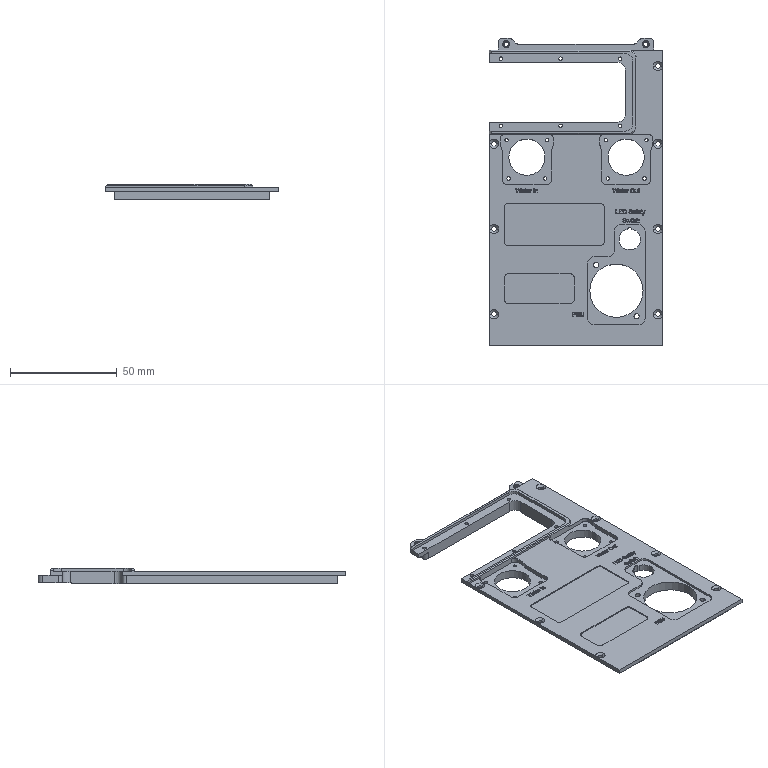NC program | NX | posted with a generic post | part box 81.5 x 144.28 x 7.5 mm
Lines 7294 to 9048 of 9048:
(CAVITY_MILL_COPY_COPY , TOOL : D2精光)
N14478 T10 M6
N14480 G54
N14482 G17 G0 G90 X29.54 Y-11.576 S6500 M3
N14484 G43 Z50. H10
N14486 Z0.
N14488 G94 G1 Z-0.2 F1200.
N14490 G3 X29.74 Y-11.376 R0.2
N14492 G1 Y-10.85
N14494 X29.602
N14496 G2 X29.301 Y-10.828 R2.1
N14498 G3 X29.076 Y-10.989 R0.2
N14500 G1 Z0.
N14502 G0 X29.54 Y-11.576 Z-0.2
N14504 G1 Z-0.4
N14506 G3 X29.74 Y-11.376 R0.2
N14508 G1 Y-10.85
N14510 X29.602
N14512 G2 X29.301 Y-10.828 R2.1
N14514 G3 X29.076 Y-10.989 R0.2
N14516 G1 Z-0.2
N14518 G0 X29.54 Y-11.576 Z-0.388
N14520 G1 Z-0.588
N14522 G3 X29.74 Y-11.376 R0.2
N14524 G1 Y-10.85
N14526 X29.602
N14528 G2 X29.301 Y-10.828 R2.1
N14530 G3 X29.076 Y-10.989 R0.2
N14532 G1 Z-0.388
N14534 G0 X29.54 Y-11.576 Z-0.575
N14536 G1 Z-0.775
N14538 G3 X29.74 Y-11.376 R0.2
N14540 G1 Y-10.85
N14542 X29.602
N14544 G2 X29.301 Y-10.828 R2.1
N14546 G3 X29.076 Y-10.989 R0.2
N14548 G1 Z-0.575
N14550 G0 X29.54 Y-11.576 Z-0.763
N14552 G1 Z-0.963
N14554 G3 X29.74 Y-11.376 R0.2
N14556 G1 Y-10.85
N14558 X29.602
N14560 G2 X29.301 Y-10.828 R2.1
N14562 G3 X29.076 Y-10.989 R0.2
N14564 G1 Z-0.763
N14566 G0 X29.54 Y-11.576 Z-0.95
N14568 G1 Z-1.15
N14570 G3 X29.74 Y-11.376 R0.2
N14572 G1 Y-10.85
N14574 X29.602
N14576 G2 X29.301 Y-10.828 R2.1
N14578 G3 X29.076 Y-10.989 R0.2
N14580 G1 Z-0.95
N14582 G0 X29.54 Y-11.576 Z-1.138
N14584 G1 Z-1.338
N14586 G3 X29.74 Y-11.376 R0.2
N14588 G1 Y-10.85
N14590 X29.602
N14592 G2 X29.301 Y-10.828 R2.1
N14594 G3 X29.076 Y-10.989 R0.2
N14596 G1 Z-1.138
N14598 G0 X29.54 Y-11.576 Z-1.325
N14600 G1 Z-1.525
N14602 G3 X29.74 Y-11.376 R0.2
N14604 G1 Y-10.85
N14606 X29.602
N14608 G2 X29.301 Y-10.828 R2.1
N14610 G3 X29.076 Y-10.989 R0.2
N14612 G1 Z-1.325
N14614 G0 X29.54 Y-11.576 Z-1.513
N14616 G1 Z-1.713
N14618 G3 X29.74 Y-11.376 R0.2
N14620 G1 Y-10.85
N14622 X29.602
N14624 G2 X29.301 Y-10.828 R2.1
N14626 G3 X29.076 Y-10.989 R0.2
N14628 G1 Z-1.513
N14630 G0 X29.54 Y-11.576 Z-1.7
N14632 G1 Z-1.9
N14634 G3 X29.74 Y-11.376 R0.2
N14636 G1 Y-10.85
N14638 X29.602
N14640 G2 X29.301 Y-10.828 R2.1
N14642 G3 X29.076 Y-10.989 R0.2
N14644 G1 Z-1.7
N14646 G0 X29.54 Y-11.576 Z-1.9
N14648 G1 Z-2.1
N14650 G3 X29.74 Y-11.376 R0.2
N14652 G1 Y-10.85
N14654 X29.602
N14656 G2 X29.301 Y-10.828 R2.1
N14658 G3 X29.076 Y-10.989 R0.2
N14660 G1 Z-1.9
N14662 G0 X29.54 Y-11.576 Z-2.1
N14664 G1 Z-2.3
N14666 G3 X29.74 Y-11.376 R0.2
N14668 G1 Y-10.85
N14670 X29.602
N14672 G2 X29.301 Y-10.828 R2.1
N14674 G3 X29.076 Y-10.989 R0.2
N14676 G1 Z-2.1
N14678 G0 X29.54 Y-11.576 Z-2.3
N14680 G1 Z-2.5
N14682 G3 X29.74 Y-11.376 R0.2
N14684 G1 Y-10.85
N14686 X29.602
N14688 G2 X29.301 Y-10.828 R2.1
N14690 G3 X29.076 Y-10.989 R0.2
N14692 G1 Z-2.3
N14694 G0 X29.54 Y-11.576 Z-2.5
N14696 G1 Z-2.7
N14698 G3 X29.74 Y-11.376 R0.2
N14700 G1 Y-10.85
N14702 X29.602
N14704 G2 X29.301 Y-10.828 R2.1
N14706 G3 X29.076 Y-10.989 R0.2
N14708 G1 Z-2.5
N14710 G0 X29.54 Y-11.576 Z-2.7
N14712 G1 Z-2.9
N14714 G3 X29.74 Y-11.376 R0.2
N14716 G1 Y-10.85
N14718 X29.602
N14720 G2 X29.301 Y-10.828 R2.1
N14722 G3 X29.076 Y-10.989 R0.2
N14724 G1 Z-2.7
N14726 G0 Z50.
N14728 X64.585 Y-10.975
N14730 Z-0.388
N14732 G1 Z-0.588
N14734 G3 X64.356 Y-10.82 R0.2
N14736 G2 X64.002 Y-10.85 R2.1
N14738 G1 X63.94
N14740 Y-11.353
N14742 G3 X64.14 Y-11.553 R0.2
N14744 G1 Z-0.388
N14746 G0 X64.585 Y-10.975 Z-0.575
N14748 G1 Z-0.775
N14750 G3 X64.356 Y-10.82 R0.2
N14752 G2 X64.002 Y-10.85 R2.1
N14754 G1 X63.94
N14756 Y-11.353
N14758 G3 X64.14 Y-11.553 R0.2
N14760 G1 Z-0.575
N14762 G0 X64.585 Y-10.975 Z-0.763
N14764 G1 Z-0.963
N14766 G3 X64.356 Y-10.82 R0.2
N14768 G2 X64.002 Y-10.85 R2.1
N14770 G1 X63.94
N14772 Y-11.353
N14774 G3 X64.14 Y-11.553 R0.2
N14776 G1 Z-0.763
N14778 G0 X64.585 Y-10.975 Z-0.95
N14780 G1 Z-1.15
N14782 G3 X64.356 Y-10.82 R0.2
N14784 G2 X64.002 Y-10.85 R2.1
N14786 G1 X63.94
N14788 Y-11.353
N14790 G3 X64.14 Y-11.553 R0.2
N14792 G1 Z-0.95
N14794 G0 X64.585 Y-10.975 Z-1.138
N14796 G1 Z-1.338
N14798 G3 X64.356 Y-10.82 R0.2
N14800 G2 X64.002 Y-10.85 R2.1
N14802 G1 X63.94
N14804 Y-11.353
N14806 G3 X64.14 Y-11.553 R0.2
N14808 G1 Z-1.138
N14810 G0 X64.585 Y-10.975 Z-1.325
N14812 G1 Z-1.525
N14814 G3 X64.356 Y-10.82 R0.2
N14816 G2 X64.002 Y-10.85 R2.1
N14818 G1 X63.94
N14820 Y-11.353
N14822 G3 X64.14 Y-11.553 R0.2
N14824 G1 Z-1.325
N14826 G0 X64.585 Y-10.975 Z-1.513
N14828 G1 Z-1.713
N14830 G3 X64.356 Y-10.82 R0.2
N14832 G2 X64.002 Y-10.85 R2.1
N14834 G1 X63.94
N14836 Y-11.353
N14838 G3 X64.14 Y-11.553 R0.2
N14840 G1 Z-1.513
N14842 G0 X64.585 Y-10.975 Z-1.7
N14844 G1 Z-1.9
N14846 G3 X64.356 Y-10.82 R0.2
N14848 G2 X64.002 Y-10.85 R2.1
N14850 G1 X63.94
N14852 Y-11.353
N14854 G3 X64.14 Y-11.553 R0.2
N14856 G1 Z-1.7
N14858 G0 X64.585 Y-10.975 Z-1.9
N14860 G1 Z-2.1
N14862 G3 X64.356 Y-10.82 R0.2
N14864 G2 X64.002 Y-10.85 R2.1
N14866 G1 X63.94
N14868 Y-11.353
N14870 G3 X64.14 Y-11.553 R0.2
N14872 G1 Z-1.9
N14874 G0 X64.585 Y-10.975 Z-2.1
N14876 G1 Z-2.3
N14878 G3 X64.356 Y-10.82 R0.2
N14880 G2 X64.002 Y-10.85 R2.1
N14882 G1 X63.94
N14884 Y-11.353
N14886 G3 X64.14 Y-11.553 R0.2
N14888 G1 Z-2.1
N14890 G0 X64.585 Y-10.975 Z-2.3
N14892 G1 Z-2.5
N14894 G3 X64.356 Y-10.82 R0.2
N14896 G2 X64.002 Y-10.85 R2.1
N14898 G1 X63.94
N14900 Y-11.353
N14902 G3 X64.14 Y-11.553 R0.2
N14904 G1 Z-2.3
N14906 G0 X64.585 Y-10.975 Z-2.5
N14908 G1 Z-2.7
N14910 G3 X64.356 Y-10.82 R0.2
N14912 G2 X64.002 Y-10.85 R2.1
N14914 G1 X63.94
N14916 Y-11.353
N14918 G3 X64.14 Y-11.553 R0.2
N14920 G1 Z-2.5
N14922 G0 X64.585 Y-10.975 Z-2.7
N14924 G1 Z-2.9
N14926 G3 X64.356 Y-10.82 R0.2
N14928 G2 X64.002 Y-10.85 R2.1
N14930 G1 X63.94
N14932 Y-11.353
N14934 G3 X64.14 Y-11.553 R0.2
N14936 G1 Z-2.7
N14938 G0 Z50.
N14940 X65.929 Y-4.022
N14942 Z-0.388
N14944 G1 Z-0.588
N14946 X65.94 Y-4.043
N14948 G3 X66.207 Y-4.135 R0.2
N14950 X66.74 Y-3.535 R1.06
N14952 G1 Y-10.965
N14954 G3 X65.407 Y-10.31 R1.06
N14956 X66.102 Y-8.75 R2.1
N14958 G1 Y-5.75
N14960 G3 X65.407 Y-4.19 R2.1
N14962 X66.207 Y-4.135 R1.06
N14964 X66.288 Y-3.846 R0.201
N14966 G1 Z-0.388
N14968 G0 X65.929 Y-4.022 Z-0.575
N14970 G1 Z-0.775
N14972 X65.94 Y-4.043
N14974 G3 X66.207 Y-4.135 R0.2
N14976 X66.74 Y-3.535 R1.06
N14978 G1 Y-10.965
N14980 G3 X65.407 Y-10.31 R1.06
N14982 X66.102 Y-8.75 R2.1
N14984 G1 Y-5.75
N14986 G3 X65.407 Y-4.19 R2.1
N14988 X66.207 Y-4.135 R1.06
N14990 X66.288 Y-3.846 R0.201
N14992 G1 Z-0.575
N14994 G0 X65.929 Y-4.022 Z-0.763
N14996 G1 Z-0.963
N14998 X65.94 Y-4.043
N15000 G3 X66.207 Y-4.135 R0.2
N15002 X66.74 Y-3.535 R1.06
N15004 G1 Y-10.965
N15006 G3 X65.407 Y-10.31 R1.06
N15008 X66.102 Y-8.75 R2.1
N15010 G1 Y-5.75
N15012 G3 X65.407 Y-4.19 R2.1
N15014 X66.207 Y-4.135 R1.06
N15016 X66.288 Y-3.846 R0.201
N15018 G1 Z-0.763
N15020 G0 X65.929 Y-4.022 Z-0.95
N15022 G1 Z-1.15
N15024 X65.94 Y-4.043
N15026 G3 X66.207 Y-4.135 R0.2
N15028 X66.74 Y-3.535 R1.06
N15030 G1 Y-10.965
N15032 G3 X65.407 Y-10.31 R1.06
N15034 X66.102 Y-8.75 R2.1
N15036 G1 Y-5.75
N15038 G3 X65.407 Y-4.19 R2.1
N15040 X66.207 Y-4.135 R1.06
N15042 X66.288 Y-3.846 R0.201
N15044 G1 Z-0.95
N15046 G0 X65.929 Y-4.022 Z-1.138
N15048 G1 Z-1.338
N15050 X65.94 Y-4.043
N15052 G3 X66.207 Y-4.135 R0.2
N15054 X66.74 Y-3.535 R1.06
N15056 G1 Y-10.965
N15058 G3 X65.407 Y-10.31 R1.06
N15060 X66.102 Y-8.75 R2.1
N15062 G1 Y-5.75
N15064 G3 X65.407 Y-4.19 R2.1
N15066 X66.207 Y-4.135 R1.06
N15068 X66.288 Y-3.846 R0.201
N15070 G1 Z-1.138
N15072 G0 X65.929 Y-4.022 Z-1.325
N15074 G1 Z-1.525
N15076 X65.94 Y-4.043
N15078 G3 X66.207 Y-4.135 R0.2
N15080 X66.74 Y-3.535 R1.06
N15082 G1 Y-10.965
N15084 G3 X65.407 Y-10.31 R1.06
N15086 X66.102 Y-8.75 R2.1
N15088 G1 Y-5.75
N15090 G3 X65.407 Y-4.19 R2.1
N15092 X66.207 Y-4.135 R1.06
N15094 X66.288 Y-3.846 R0.201
N15096 G1 Z-1.325
N15098 G0 X65.929 Y-4.022 Z-1.513
N15100 G1 Z-1.713
N15102 X65.94 Y-4.043
N15104 G3 X66.207 Y-4.135 R0.2
N15106 X66.74 Y-3.535 R1.06
N15108 G1 Y-10.965
N15110 G3 X65.407 Y-10.31 R1.06
N15112 X66.102 Y-8.75 R2.1
N15114 G1 Y-5.75
N15116 G3 X65.407 Y-4.19 R2.1
N15118 X66.207 Y-4.135 R1.06
N15120 X66.288 Y-3.846 R0.201
N15122 G1 Z-1.513
N15124 G0 X65.929 Y-4.022 Z-1.7
N15126 G1 Z-1.9
N15128 X65.94 Y-4.043
N15130 G3 X66.207 Y-4.135 R0.2
N15132 X66.74 Y-3.535 R1.06
N15134 G1 Y-10.965
N15136 G3 X65.407 Y-10.31 R1.06
N15138 X66.102 Y-8.75 R2.1
N15140 G1 Y-5.75
N15142 G3 X65.407 Y-4.19 R2.1
N15144 X66.207 Y-4.135 R1.06
N15146 X66.288 Y-3.846 R0.201
N15148 G1 Z-1.7
N15150 G0 X65.929 Y-4.022 Z-1.9
N15152 G1 Z-2.1
N15154 X65.94 Y-4.043
N15156 G3 X66.207 Y-4.135 R0.2
N15158 X66.74 Y-3.535 R1.06
N15160 G1 Y-10.965
N15162 G3 X65.407 Y-10.31 R1.06
N15164 X66.102 Y-8.75 R2.1
N15166 G1 Y-5.75
N15168 G3 X65.407 Y-4.19 R2.1
N15170 X66.207 Y-4.135 R1.06
N15172 X66.288 Y-3.846 R0.201
N15174 G1 Z-1.9
N15176 G0 X65.929 Y-4.022 Z-2.1
N15178 G1 Z-2.3
N15180 X65.94 Y-4.043
N15182 G3 X66.207 Y-4.135 R0.2
N15184 X66.74 Y-3.535 R1.06
N15186 G1 Y-10.965
N15188 G3 X65.407 Y-10.31 R1.06
N15190 X66.102 Y-8.75 R2.1
N15192 G1 Y-5.75
N15194 G3 X65.407 Y-4.19 R2.1
N15196 X66.207 Y-4.135 R1.06
N15198 X66.288 Y-3.846 R0.201
N15200 G1 Z-2.1
N15202 G0 X65.929 Y-4.022 Z-2.3
N15204 G1 Z-2.5
N15206 X65.94 Y-4.043
N15208 G3 X66.207 Y-4.135 R0.2
N15210 X66.74 Y-3.535 R1.06
N15212 G1 Y-10.965
N15214 G3 X65.407 Y-10.31 R1.06
N15216 X66.102 Y-8.75 R2.1
N15218 G1 Y-5.75
N15220 G3 X65.407 Y-4.19 R2.1
N15222 X66.207 Y-4.135 R1.06
N15224 X66.288 Y-3.846 R0.201
N15226 G1 Z-2.3
N15228 G0 X65.929 Y-4.022 Z-2.5
N15230 G1 Z-2.7
N15232 X65.94 Y-4.043
N15234 G3 X66.207 Y-4.135 R0.2
N15236 X66.74 Y-3.535 R1.06
N15238 G1 Y-10.965
N15240 G3 X65.407 Y-10.31 R1.06
N15242 X66.102 Y-8.75 R2.1
N15244 G1 Y-5.75
N15246 G3 X65.407 Y-4.19 R2.1
N15248 X66.207 Y-4.135 R1.06
N15250 X66.288 Y-3.846 R0.201
N15252 G1 Z-2.5
N15254 G0 X65.929 Y-4.022 Z-2.7
N15256 G1 Z-2.9
N15258 X65.94 Y-4.043
N15260 G3 X66.207 Y-4.135 R0.2
N15262 X66.74 Y-3.535 R1.06
N15264 G1 Y-10.965
N15266 G3 X65.407 Y-10.31 R1.06
N15268 X66.102 Y-8.75 R2.1
N15270 G1 Y-5.75
N15272 G3 X65.407 Y-4.19 R2.1
N15274 X66.207 Y-4.135 R1.06
N15276 X66.288 Y-3.846 R0.201
N15278 G1 Z-2.7
N15280 G0 X64.14 Y-2.947 Z-0.388
N15282 G1 Z-0.588
N15284 G3 X63.94 Y-3.147 R0.2
N15286 G1 Y-3.65
N15288 X64.002
N15290 G2 X64.356 Y-3.68 R2.1
N15292 G3 X64.585 Y-3.525 R0.2
N15294 G1 Z-0.388
N15296 G0 X64.14 Y-2.947 Z-0.575
N15298 G1 Z-0.775
N15300 G3 X63.94 Y-3.147 R0.2
N15302 G1 Y-3.65
N15304 X64.002
N15306 G2 X64.356 Y-3.68 R2.1
N15308 G3 X64.585 Y-3.525 R0.2
N15310 G1 Z-0.575
N15312 G0 X64.14 Y-2.947 Z-0.763
N15314 G1 Z-0.963
N15316 G3 X63.94 Y-3.147 R0.2
N15318 G1 Y-3.65
N15320 X64.002
N15322 G2 X64.356 Y-3.68 R2.1
N15324 G3 X64.585 Y-3.525 R0.2
N15326 G1 Z-0.763
N15328 G0 X64.14 Y-2.947 Z-0.95
N15330 G1 Z-1.15
N15332 G3 X63.94 Y-3.147 R0.2
N15334 G1 Y-3.65
N15336 X64.002
N15338 G2 X64.356 Y-3.68 R2.1
N15340 G3 X64.585 Y-3.525 R0.2
N15342 G1 Z-0.95
N15344 G0 X64.14 Y-2.947 Z-1.138
N15346 G1 Z-1.338
N15348 G3 X63.94 Y-3.147 R0.2
N15350 G1 Y-3.65
N15352 X64.002
N15354 G2 X64.356 Y-3.68 R2.1
N15356 G3 X64.585 Y-3.525 R0.2
N15358 G1 Z-1.138
N15360 G0 X64.14 Y-2.947 Z-1.325
N15362 G1 Z-1.525
N15364 G3 X63.94 Y-3.147 R0.2
N15366 G1 Y-3.65
N15368 X64.002
N15370 G2 X64.356 Y-3.68 R2.1
N15372 G3 X64.585 Y-3.525 R0.2
N15374 G1 Z-1.325
N15376 G0 X64.14 Y-2.947 Z-1.513
N15378 G1 Z-1.713
N15380 G3 X63.94 Y-3.147 R0.2
N15382 G1 Y-3.65
N15384 X64.002
N15386 G2 X64.356 Y-3.68 R2.1
N15388 G3 X64.585 Y-3.525 R0.2
N15390 G1 Z-1.513
N15392 G0 X64.14 Y-2.947 Z-1.7
N15394 G1 Z-1.9
N15396 G3 X63.94 Y-3.147 R0.2
N15398 G1 Y-3.65
N15400 X64.002
N15402 G2 X64.356 Y-3.68 R2.1
N15404 G3 X64.585 Y-3.525 R0.2
N15406 G1 Z-1.7
N15408 G0 X64.14 Y-2.947 Z-1.9
N15410 G1 Z-2.1
N15412 G3 X63.94 Y-3.147 R0.2
N15414 G1 Y-3.65
N15416 X64.002
N15418 G2 X64.356 Y-3.68 R2.1
N15420 G3 X64.585 Y-3.525 R0.2
N15422 G1 Z-1.9
N15424 G0 X64.14 Y-2.947 Z-2.1
N15426 G1 Z-2.3
N15428 G3 X63.94 Y-3.147 R0.2
N15430 G1 Y-3.65
N15432 X64.002
N15434 G2 X64.356 Y-3.68 R2.1
N15436 G3 X64.585 Y-3.525 R0.2
N15438 G1 Z-2.1
N15440 G0 X64.14 Y-2.947 Z-2.3
N15442 G1 Z-2.5
N15444 G3 X63.94 Y-3.147 R0.2
N15446 G1 Y-3.65
N15448 X64.002
N15450 G2 X64.356 Y-3.68 R2.1
N15452 G3 X64.585 Y-3.525 R0.2
N15454 G1 Z-2.3
N15456 G0 X64.14 Y-2.947 Z-2.5
N15458 G1 Z-2.7
N15460 G3 X63.94 Y-3.147 R0.2
N15462 G1 Y-3.65
N15464 X64.002
N15466 G2 X64.356 Y-3.68 R2.1
N15468 G3 X64.585 Y-3.525 R0.2
N15470 G1 Z-2.5
N15472 G0 X64.14 Y-2.947 Z-2.7
N15474 G1 Z-2.9
N15476 G3 X63.94 Y-3.147 R0.2
N15478 G1 Y-3.65
N15480 X64.002
N15482 G2 X64.356 Y-3.68 R2.1
N15484 G3 X64.585 Y-3.525 R0.2
N15486 G1 Z-2.7
N15488 G0 X66.288 Y17.346 Z-0.388
N15490 G1 Z-0.588
N15492 X66.299 Y17.367
N15494 G3 X66.207 Y17.635 R0.2
N15496 X65.407 Y17.69 R1.06
N15498 X66.102 Y19.25 R2.1
N15500 G1 Y22.25
N15502 G3 X65.407 Y23.81 R2.1
N15504 X66.74 Y24.465 R1.06
N15506 G1 Y17.035
N15508 G3 X66.207 Y17.635 R1.06
N15510 X65.929 Y17.522 R0.201
N15512 G1 Z-0.388
N15514 G0 X66.288 Y17.346 Z-0.575
N15516 G1 Z-0.775
N15518 X66.299 Y17.367
N15520 G3 X66.207 Y17.635 R0.2
N15522 X65.407 Y17.69 R1.06
N15524 X66.102 Y19.25 R2.1
N15526 G1 Y22.25
N15528 G3 X65.407 Y23.81 R2.1
N15530 X66.74 Y24.465 R1.06
N15532 G1 Y17.035
N15534 G3 X66.207 Y17.635 R1.06
N15536 X65.929 Y17.522 R0.201
N15538 G1 Z-0.575
N15540 G0 X66.288 Y17.346 Z-0.763
N15542 G1 Z-0.963
N15544 X66.299 Y17.367
N15546 G3 X66.207 Y17.635 R0.2
N15548 X65.407 Y17.69 R1.06
N15550 X66.102 Y19.25 R2.1
N15552 G1 Y22.25
N15554 G3 X65.407 Y23.81 R2.1
N15556 X66.74 Y24.465 R1.06
N15558 G1 Y17.035
N15560 G3 X66.207 Y17.635 R1.06
N15562 X65.929 Y17.522 R0.201
N15564 G1 Z-0.763
N15566 G0 X66.288 Y17.346 Z-0.95
N15568 G1 Z-1.15
N15570 X66.299 Y17.367
N15572 G3 X66.207 Y17.635 R0.2
N15574 X65.407 Y17.69 R1.06
N15576 X66.102 Y19.25 R2.1
N15578 G1 Y22.25
N15580 G3 X65.407 Y23.81 R2.1
N15582 X66.74 Y24.465 R1.06
N15584 G1 Y17.035
N15586 G3 X66.207 Y17.635 R1.06
N15588 X65.929 Y17.522 R0.201
N15590 G1 Z-0.95
N15592 G0 X66.288 Y17.346 Z-1.138
N15594 G1 Z-1.338
N15596 X66.299 Y17.367
N15598 G3 X66.207 Y17.635 R0.2
N15600 X65.407 Y17.69 R1.06
N15602 X66.102 Y19.25 R2.1
N15604 G1 Y22.25
N15606 G3 X65.407 Y23.81 R2.1
N15608 X66.74 Y24.465 R1.06
N15610 G1 Y17.035
N15612 G3 X66.207 Y17.635 R1.06
N15614 X65.929 Y17.522 R0.201
N15616 G1 Z-1.138
N15618 G0 X66.288 Y17.346 Z-1.325
N15620 G1 Z-1.525
N15622 X66.299 Y17.367
N15624 G3 X66.207 Y17.635 R0.2
N15626 X65.407 Y17.69 R1.06
N15628 X66.102 Y19.25 R2.1
N15630 G1 Y22.25
N15632 G3 X65.407 Y23.81 R2.1
N15634 X66.74 Y24.465 R1.06
N15636 G1 Y17.035
N15638 G3 X66.207 Y17.635 R1.06
N15640 X65.929 Y17.522 R0.201
N15642 G1 Z-1.325
N15644 G0 X66.288 Y17.346 Z-1.513
N15646 G1 Z-1.713
N15648 X66.299 Y17.367
N15650 G3 X66.207 Y17.635 R0.2
N15652 X65.407 Y17.69 R1.06
N15654 X66.102 Y19.25 R2.1
N15656 G1 Y22.25
N15658 G3 X65.407 Y23.81 R2.1
N15660 X66.74 Y24.465 R1.06
N15662 G1 Y17.035
N15664 G3 X66.207 Y17.635 R1.06
N15666 X65.929 Y17.522 R0.201
N15668 G1 Z-1.513
N15670 G0 X66.288 Y17.346 Z-1.7
N15672 G1 Z-1.9
N15674 X66.299 Y17.367
N15676 G3 X66.207 Y17.635 R0.2
N15678 X65.407 Y17.69 R1.06
N15680 X66.102 Y19.25 R2.1
N15682 G1 Y22.25
N15684 G3 X65.407 Y23.81 R2.1
N15686 X66.74 Y24.465 R1.06
N15688 G1 Y17.035
N15690 G3 X66.207 Y17.635 R1.06
N15692 X65.929 Y17.522 R0.201
N15694 G1 Z-1.7
N15696 G0 X66.288 Y17.346 Z-1.9
N15698 G1 Z-2.1
N15700 X66.299 Y17.367
N15702 G3 X66.207 Y17.635 R0.2
N15704 X65.407 Y17.69 R1.06
N15706 X66.102 Y19.25 R2.1
N15708 G1 Y22.25
N15710 G3 X65.407 Y23.81 R2.1
N15712 X66.74 Y24.465 R1.06
N15714 G1 Y17.035
N15716 G3 X66.207 Y17.635 R1.06
N15718 X65.929 Y17.522 R0.201
N15720 G1 Z-1.9
N15722 G0 X66.288 Y17.346 Z-2.1
N15724 G1 Z-2.3
N15726 X66.299 Y17.367
N15728 G3 X66.207 Y17.635 R0.2
N15730 X65.407 Y17.69 R1.06
N15732 X66.102 Y19.25 R2.1
N15734 G1 Y22.25
N15736 G3 X65.407 Y23.81 R2.1
N15738 X66.74 Y24.465 R1.06
N15740 G1 Y17.035
N15742 G3 X66.207 Y17.635 R1.06
N15744 X65.929 Y17.522 R0.201
N15746 G1 Z-2.1
N15748 G0 X66.288 Y17.346 Z-2.3
N15750 G1 Z-2.5
N15752 X66.299 Y17.367
N15754 G3 X66.207 Y17.635 R0.2
N15756 X65.407 Y17.69 R1.06
N15758 X66.102 Y19.25 R2.1
N15760 G1 Y22.25
N15762 G3 X65.407 Y23.81 R2.1
N15764 X66.74 Y24.465 R1.06
N15766 G1 Y17.035
N15768 G3 X66.207 Y17.635 R1.06
N15770 X65.929 Y17.522 R0.201
N15772 G1 Z-2.3
N15774 G0 X66.288 Y17.346 Z-2.5
N15776 G1 Z-2.7
N15778 X66.299 Y17.367
N15780 G3 X66.207 Y17.635 R0.2
N15782 X65.407 Y17.69 R1.06
N15784 X66.102 Y19.25 R2.1
N15786 G1 Y22.25
N15788 G3 X65.407 Y23.81 R2.1
N15790 X66.74 Y24.465 R1.06
N15792 G1 Y17.035
N15794 G3 X66.207 Y17.635 R1.06
N15796 X65.929 Y17.522 R0.201
N15798 G1 Z-2.5
N15800 G0 X66.288 Y17.346 Z-2.7
N15802 G1 Z-2.9
N15804 X66.299 Y17.367
N15806 G3 X66.207 Y17.635 R0.2
N15808 X65.407 Y17.69 R1.06
N15810 X66.102 Y19.25 R2.1
N15812 G1 Y22.25
N15814 G3 X65.407 Y23.81 R2.1
N15816 X66.74 Y24.465 R1.06
N15818 G1 Y17.035
N15820 G3 X66.207 Y17.635 R1.06
N15822 X65.929 Y17.522 R0.201
N15824 G1 Z-2.7
N15826 G0 Z50.
N15828 X61.902 Y25.192
N15830 Z-0.388
N15832 G1 Z-0.588
N15834 G3 X61.702 Y24.992 R0.2
N15836 G1 Y24.35
N15838 X62.348
N15840 G3 X62.548 Y24.55 R0.2
N15842 G1 Z-0.388
N15844 G0 X61.902 Y25.192 Z-0.575
N15846 G1 Z-0.775
N15848 G3 X61.702 Y24.992 R0.2
N15850 G1 Y24.35
N15852 X62.348
N15854 G3 X62.548 Y24.55 R0.2
N15856 G1 Z-0.575
N15858 G0 X61.902 Y25.192 Z-0.763
N15860 G1 Z-0.963
N15862 G3 X61.702 Y24.992 R0.2
N15864 G1 Y24.35
N15866 X62.348
N15868 G3 X62.548 Y24.55 R0.2
N15870 G1 Z-0.763
N15872 G0 X61.902 Y25.192 Z-0.95
N15874 G1 Z-1.15
N15876 G3 X61.702 Y24.992 R0.2
N15878 G1 Y24.35
N15880 X62.348
N15882 G3 X62.548 Y24.55 R0.2
N15884 G1 Z-0.95
N15886 G0 X61.902 Y25.192 Z-1.138
N15888 G1 Z-1.338
N15890 G3 X61.702 Y24.992 R0.2
N15892 G1 Y24.35
N15894 X62.348
N15896 G3 X62.548 Y24.55 R0.2
N15898 G1 Z-1.138
N15900 G0 X61.902 Y25.192 Z-1.325
N15902 G1 Z-1.525
N15904 G3 X61.702 Y24.992 R0.2
N15906 G1 Y24.35
N15908 X62.348
N15910 G3 X62.548 Y24.55 R0.2
N15912 G1 Z-1.325
N15914 G0 X61.902 Y25.192 Z-1.513
N15916 G1 Z-1.713
N15918 G3 X61.702 Y24.992 R0.2
N15920 G1 Y24.35
N15922 X62.348
N15924 G3 X62.548 Y24.55 R0.2
N15926 G1 Z-1.513
N15928 G0 X61.902 Y25.192 Z-1.7
N15930 G1 Z-1.9
N15932 G3 X61.702 Y24.992 R0.2
N15934 G1 Y24.35
N15936 X62.348
N15938 G3 X62.548 Y24.55 R0.2
N15940 G1 Z-1.7
N15942 G0 X61.902 Y25.192 Z-1.9
N15944 G1 Z-2.1
N15946 G3 X61.702 Y24.992 R0.2
N15948 G1 Y24.35
N15950 X62.348
N15952 G3 X62.548 Y24.55 R0.2
N15954 G1 Z-1.9
N15956 G0 X61.902 Y25.192 Z-2.1
N15958 G1 Z-2.3
N15960 G3 X61.702 Y24.992 R0.2
N15962 G1 Y24.35
N15964 X62.348
N15966 G3 X62.548 Y24.55 R0.2
N15968 G1 Z-2.1
N15970 G0 X61.902 Y25.192 Z-2.3
N15972 G1 Z-2.5
N15974 G3 X61.702 Y24.992 R0.2
N15976 G1 Y24.35
N15978 X62.348
N15980 G3 X62.548 Y24.55 R0.2
N15982 G1 Z-2.3
N15984 G0 X61.902 Y25.192 Z-2.5
N15986 G1 Z-2.7
N15988 G3 X61.702 Y24.992 R0.2
N15990 G1 Y24.35
N15992 X62.348
N15994 G3 X62.548 Y24.55 R0.2
N15996 G1 Z-2.5
N15998 G0 X61.902 Y25.192 Z-2.7
N16000 G1 Z-2.9
N16002 G3 X61.702 Y24.992 R0.2
N16004 G1 Y24.35
N16006 X62.348
N16008 G3 X62.548 Y24.55 R0.2
N16010 G1 Z-2.7
N16012 G0 Z50.
N16014 X64.585 Y17.025
N16016 Z-0.388
N16018 G1 Z-0.588
N16020 G3 X64.356 Y17.18 R0.2
N16022 G2 X64.002 Y17.15 R2.1
N16024 G1 X63.94
N16026 Y16.647
N16028 G3 X64.14 Y16.447 R0.2
N16030 G1 Z-0.388
N16032 G0 X64.585 Y17.025 Z-0.575
N16034 G1 Z-0.775
N16036 G3 X64.356 Y17.18 R0.2
N16038 G2 X64.002 Y17.15 R2.1
N16040 G1 X63.94
N16042 Y16.647
N16044 G3 X64.14 Y16.447 R0.2
N16046 G1 Z-0.575
N16048 G0 X64.585 Y17.025 Z-0.763
N16050 G1 Z-0.963
N16052 G3 X64.356 Y17.18 R0.2
N16054 G2 X64.002 Y17.15 R2.1
N16056 G1 X63.94
N16058 Y16.647
N16060 G3 X64.14 Y16.447 R0.2
N16062 G1 Z-0.763
N16064 G0 X64.585 Y17.025 Z-0.95
N16066 G1 Z-1.15
N16068 G3 X64.356 Y17.18 R0.2
N16070 G2 X64.002 Y17.15 R2.1
N16072 G1 X63.94
N16074 Y16.647
N16076 G3 X64.14 Y16.447 R0.2
N16078 G1 Z-0.95
N16080 G0 X64.585 Y17.025 Z-1.138
N16082 G1 Z-1.338
N16084 G3 X64.356 Y17.18 R0.2
N16086 G2 X64.002 Y17.15 R2.1
N16088 G1 X63.94
N16090 Y16.647
N16092 G3 X64.14 Y16.447 R0.2
N16094 G1 Z-1.138
N16096 G0 X64.585 Y17.025 Z-1.325
N16098 G1 Z-1.525
N16100 G3 X64.356 Y17.18 R0.2
N16102 G2 X64.002 Y17.15 R2.1
N16104 G1 X63.94
N16106 Y16.647
N16108 G3 X64.14 Y16.447 R0.2
N16110 G1 Z-1.325
N16112 G0 X64.585 Y17.025 Z-1.513
N16114 G1 Z-1.713
N16116 G3 X64.356 Y17.18 R0.2
N16118 G2 X64.002 Y17.15 R2.1
N16120 G1 X63.94
N16122 Y16.647
N16124 G3 X64.14 Y16.447 R0.2
N16126 G1 Z-1.513
N16128 G0 X64.585 Y17.025 Z-1.7
N16130 G1 Z-1.9
N16132 G3 X64.356 Y17.18 R0.2
N16134 G2 X64.002 Y17.15 R2.1
N16136 G1 X63.94
N16138 Y16.647
N16140 G3 X64.14 Y16.447 R0.2
N16142 G1 Z-1.7
N16144 G0 X64.585 Y17.025 Z-1.9
N16146 G1 Z-2.1
N16148 G3 X64.356 Y17.18 R0.2
N16150 G2 X64.002 Y17.15 R2.1
N16152 G1 X63.94
N16154 Y16.647
N16156 G3 X64.14 Y16.447 R0.2
N16158 G1 Z-1.9
N16160 G0 X64.585 Y17.025 Z-2.1
N16162 G1 Z-2.3
N16164 G3 X64.356 Y17.18 R0.2
N16166 G2 X64.002 Y17.15 R2.1
N16168 G1 X63.94
N16170 Y16.647
N16172 G3 X64.14 Y16.447 R0.2
N16174 G1 Z-2.1
N16176 G0 X64.585 Y17.025 Z-2.3
N16178 G1 Z-2.5
N16180 G3 X64.356 Y17.18 R0.2
N16182 G2 X64.002 Y17.15 R2.1
N16184 G1 X63.94
N16186 Y16.647
N16188 G3 X64.14 Y16.447 R0.2
N16190 G1 Z-2.3
N16192 G0 X64.585 Y17.025 Z-2.5
N16194 G1 Z-2.7
N16196 G3 X64.356 Y17.18 R0.2
N16198 G2 X64.002 Y17.15 R2.1
N16200 G1 X63.94
N16202 Y16.647
N16204 G3 X64.14 Y16.447 R0.2
N16206 G1 Z-2.5
N16208 G0 X64.585 Y17.025 Z-2.7
N16210 G1 Z-2.9
N16212 G3 X64.356 Y17.18 R0.2
N16214 G2 X64.002 Y17.15 R2.1
N16216 G1 X63.94
N16218 Y16.647
N16220 G3 X64.14 Y16.447 R0.2
N16222 G1 Z-2.7
N16224 G0 Z50.
N16226 X29.076 Y-3.511
N16228 Z0.
N16230 G1 Z-0.2
N16232 G3 X29.301 Y-3.672 R0.2
N16234 G2 X29.602 Y-3.65 R2.1
N16236 G1 X29.74
N16238 Y-3.124
N16240 G3 X29.54 Y-2.924 R0.2
N16242 G1 Z0.
N16244 G0 X29.076 Y-3.511 Z-0.2
N16246 G1 Z-0.4
N16248 G3 X29.301 Y-3.672 R0.2
N16250 G2 X29.602 Y-3.65 R2.1
N16252 G1 X29.74
N16254 Y-3.124
N16256 G3 X29.54 Y-2.924 R0.2
N16258 G1 Z-0.2
N16260 G0 X29.076 Y-3.511 Z-0.388
N16262 G1 Z-0.588
N16264 G3 X29.301 Y-3.672 R0.2
N16266 G2 X29.602 Y-3.65 R2.1
N16268 G1 X29.74
N16270 Y-3.124
N16272 G3 X29.54 Y-2.924 R0.2
N16274 G1 Z-0.388
N16276 G0 X29.076 Y-3.511 Z-0.575
N16278 G1 Z-0.775
N16280 G3 X29.301 Y-3.672 R0.2
N16282 G2 X29.602 Y-3.65 R2.1
N16284 G1 X29.74
N16286 Y-3.124
N16288 G3 X29.54 Y-2.924 R0.2
N16290 G1 Z-0.575
N16292 G0 X29.076 Y-3.511 Z-0.763
N16294 G1 Z-0.963
N16296 G3 X29.301 Y-3.672 R0.2
N16298 G2 X29.602 Y-3.65 R2.1
N16300 G1 X29.74
N16302 Y-3.124
N16304 G3 X29.54 Y-2.924 R0.2
N16306 G1 Z-0.763
N16308 G0 X29.076 Y-3.511 Z-0.95
N16310 G1 Z-1.15
N16312 G3 X29.301 Y-3.672 R0.2
N16314 G2 X29.602 Y-3.65 R2.1
N16316 G1 X29.74
N16318 Y-3.124
N16320 G3 X29.54 Y-2.924 R0.2
N16322 G1 Z-0.95
N16324 G0 X29.076 Y-3.511 Z-1.138
N16326 G1 Z-1.338
N16328 G3 X29.301 Y-3.672 R0.2
N16330 G2 X29.602 Y-3.65 R2.1
N16332 G1 X29.74
N16334 Y-3.124
N16336 G3 X29.54 Y-2.924 R0.2
N16338 G1 Z-1.138
N16340 G0 X29.076 Y-3.511 Z-1.325
N16342 G1 Z-1.525
N16344 G3 X29.301 Y-3.672 R0.2
N16346 G2 X29.602 Y-3.65 R2.1
N16348 G1 X29.74
N16350 Y-3.124
N16352 G3 X29.54 Y-2.924 R0.2
N16354 G1 Z-1.325
N16356 G0 X29.076 Y-3.511 Z-1.513
N16358 G1 Z-1.713
N16360 G3 X29.301 Y-3.672 R0.2
N16362 G2 X29.602 Y-3.65 R2.1
N16364 G1 X29.74
N16366 Y-3.124
N16368 G3 X29.54 Y-2.924 R0.2
N16370 G1 Z-1.513
N16372 G0 X29.076 Y-3.511 Z-1.7
N16374 G1 Z-1.9
N16376 G3 X29.301 Y-3.672 R0.2
N16378 G2 X29.602 Y-3.65 R2.1
N16380 G1 X29.74
N16382 Y-3.124
N16384 G3 X29.54 Y-2.924 R0.2
N16386 G1 Z-1.7
N16388 G0 X29.076 Y-3.511 Z-1.9
N16390 G1 Z-2.1
N16392 G3 X29.301 Y-3.672 R0.2
N16394 G2 X29.602 Y-3.65 R2.1
N16396 G1 X29.74
N16398 Y-3.124
N16400 G3 X29.54 Y-2.924 R0.2
N16402 G1 Z-1.9
N16404 G0 X29.076 Y-3.511 Z-2.1
N16406 G1 Z-2.3
N16408 G3 X29.301 Y-3.672 R0.2
N16410 G2 X29.602 Y-3.65 R2.1
N16412 G1 X29.74
N16414 Y-3.124
N16416 G3 X29.54 Y-2.924 R0.2
N16418 G1 Z-2.1
N16420 G0 X29.076 Y-3.511 Z-2.3
N16422 G1 Z-2.5
N16424 G3 X29.301 Y-3.672 R0.2
N16426 G2 X29.602 Y-3.65 R2.1
N16428 G1 X29.74
N16430 Y-3.124
N16432 G3 X29.54 Y-2.924 R0.2
N16434 G1 Z-2.3
N16436 G0 X29.076 Y-3.511 Z-2.5
N16438 G1 Z-2.7
N16440 G3 X29.301 Y-3.672 R0.2
N16442 G2 X29.602 Y-3.65 R2.1
N16444 G1 X29.74
N16446 Y-3.124
N16448 G3 X29.54 Y-2.924 R0.2
N16450 G1 Z-2.5
N16452 G0 X29.076 Y-3.511 Z-2.7
N16454 G1 Z-2.9
N16456 G3 X29.301 Y-3.672 R0.2
N16458 G2 X29.602 Y-3.65 R2.1
N16460 G1 X29.74
N16462 Y-3.124
N16464 G3 X29.54 Y-2.924 R0.2
N16466 G1 Z-2.7
N16468 G0 Z50.
(CAVITY_MILL_COPY_1_COPY , TOOL : D2精光)
N16470 X66.44 Y0.676 S5500
N16472 Z-2.5
N16474 G1 Z-3. F800.
N16476 G41 X66.64 Y0.675 D10
N16478 G3 X66.84 Y0.875 R0.2
N16480 G1 Y32.5
N16482 G3 X65.84 Y33.5 R1.
N16484 G1 X28.54
N16486 G3 X27.54 Y32.5 R1.
N16488 G1 Y27.25
N16490 G3 X28.54 Y26.25 R1.
N16492 G1 X60.602
N16494 G2 X61.602 Y25.25 R1.
N16496 G1 Y24.25
N16498 X64.002
N16500 G2 X66.002 Y22.25 R2.
N16502 G1 Y19.25
N16504 G2 X64.002 Y17.25 R2.
N16506 G1 X63.84
N16508 Y-3.75
N16510 X64.002
N16512 G2 X66.002 Y-5.75 R2.
N16514 G1 Y-8.75
N16516 G2 X64.002 Y-10.75 R2.
N16518 G1 X63.84
N16520 Y-30.75
N16522 G3 X64.84 Y-31.75 R1.
N16524 G1 X65.84
N16526 G3 X66.84 Y-30.75 R1.
N16528 G1 Y0.875
N16530 G3 X66.64 Y1.075 R0.2
N16532 G40
N16534 G1 X66.44 Y1.074
N16536 Z-2.5
N16538 G0 Z50.
N16540 X-1.084 Y-10.15
N16542 Z-2.5
N16544 G1 Z-3.
N16546 G41 X-1.085 Y-10.35
N16548 G3 X-0.885 Y-10.55 R0.2
N16550 G1 X24.54
N16552 G2 X27.54 Y-13.55 R3.
N16554 G1 Y-31.1
N16556 G3 X28.69 Y-32.25 R1.15
N16558 X29.84 Y-31.1 R1.15
N16560 G1 Y-10.75
N16562 X29.602
N16564 G2 X27.602 Y-8.75 R2.
N16566 G1 Y-5.75
N16568 G2 X29.602 Y-3.75 R2.
N16570 G1 X29.84
N16572 Y16.1
N16574 G3 X28.69 Y17.25 R1.15
N16576 X27.54 Y16.1 R1.15
N16578 G1 Y13.85
N16580 G2 X24.54 Y10.85 R3.
N16582 G1 X-26.31
N16584 G3 X-27.31 Y9.85 R1.
N16586 G1 Y-9.55
N16588 G3 X-26.31 Y-10.55 R1.
N16590 G1 X-0.885
N16592 G3 X-0.685 Y-10.35 R0.2
N16594 G40
N16596 G1 X-0.686 Y-10.15
N16598 Z-2.5
N16600 G0 Z50.
(CAVITY_MILL_COPY_1_COPY_COPY_COPY , TOOL : D2精光)
N16602 X66.44 Y0.676
N16604 Z-2.5
N16606 G1 Z-3. F300.
N16608 G41 X66.64 Y0.675
N16610 G3 X66.84 Y0.875 R0.2
N16612 G1 Y32.5
N16614 G3 X65.84 Y33.5 R1.
N16616 G1 X28.54
N16618 G3 X27.54 Y32.5 R1.
N16620 G1 Y27.25
N16622 G3 X28.54 Y26.25 R1.
N16624 G1 X60.602
N16626 G2 X61.602 Y25.25 R1.
N16628 G1 Y24.25
N16630 X64.002
N16632 G2 X66.002 Y22.25 R2.
N16634 G1 Y19.25
N16636 G2 X64.002 Y17.25 R2.
N16638 G1 X63.84
N16640 Y-3.75
N16642 X64.002
N16644 G2 X66.002 Y-5.75 R2.
N16646 G1 Y-8.75
N16648 G2 X64.002 Y-10.75 R2.
N16650 G1 X63.84
N16652 Y-30.75
N16654 G3 X64.84 Y-31.75 R1.
N16656 G1 X65.84
N16658 G3 X66.84 Y-30.75 R1.
N16660 G1 Y0.875
N16662 G3 X66.64 Y1.075 R0.2
N16664 G40
N16666 G1 X66.44 Y1.074
N16668 Z-2.5
N16670 G0 Z50.
N16672 X-1.084 Y-10.15
N16674 Z-2.5
N16676 G1 Z-3.
N16678 G41 X-1.085 Y-10.35
N16680 G3 X-0.885 Y-10.55 R0.2
N16682 G1 X24.54
N16684 G2 X27.54 Y-13.55 R3.
N16686 G1 Y-31.1
N16688 G3 X28.69 Y-32.25 R1.15
N16690 X29.84 Y-31.1 R1.15
N16692 G1 Y-10.75
N16694 X29.602
N16696 G2 X27.602 Y-8.75 R2.
N16698 G1 Y-5.75
N16700 G2 X29.602 Y-3.75 R2.
N16702 G1 X29.84
N16704 Y16.1
N16706 G3 X28.69 Y17.25 R1.15
N16708 X27.54 Y16.1 R1.15
N16710 G1 Y13.85
N16712 G2 X24.54 Y10.85 R3.
N16714 G1 X-26.31
N16716 G3 X-27.31 Y9.85 R1.
N16718 G1 Y-9.55
N16720 G3 X-26.31 Y-10.55 R1.
N16722 G1 X-0.885
N16724 G3 X-0.685 Y-10.35 R0.2
N16726 G40
N16728 G1 X-0.686 Y-10.15
N16730 Z-2.5
N16732 G0 Z50.
N16734 M5
(PLANAR_MILL_COPY_COPY_1_COPY_COPY_COPY_1_COPY_COPY_1_COPY_COPY_1_COPY , TOOL :)
N16736 T12 M6
N16738 G54
N16740 G17 G0 G90 X-20.458 Y22.801 S4500 M3
N16742 G43 Z50. H12
N16744 Z-0.3
N16746 G94 G1 Z-2.3 F600.
N16748 X-20.174 Y22.616
N16750 G3 X-18.791 Y22.908 R1.
N16752 X-18.459 Y23.523 R4.2
N16754 G1 Y24.2
N16756 G2 X-17.659 Y25. R0.8
N16758 G3 X-17.459 Y25.2 R0.2
N16760 X-17.659 Y25.4 R0.2
N16762 G2 X-18.459 Y26.2 R0.8
N16764 G1 Y26.877
N16766 G3 X-18.791 Y27.492 R4.2
N16768 X-20.174 Y27.784 R1.
N16770 G1 X-20.458 Y27.599
N16772 Z-0.3
N16774 G0 Z1.
N16776 Y22.801
N16778 Z-0.6
N16780 G1 Z-2.6
N16782 X-20.174 Y22.616
N16784 G3 X-18.791 Y22.908 R1.
N16786 X-18.459 Y23.523 R4.2
N16788 G1 Y24.2
N16790 G2 X-17.659 Y25. R0.8
N16792 G3 X-17.459 Y25.2 R0.2
N16794 X-17.659 Y25.4 R0.2
N16796 G2 X-18.459 Y26.2 R0.8
N16798 G1 Y26.877
N16800 G3 X-18.791 Y27.492 R4.2
N16802 X-20.174 Y27.784 R1.
N16804 G1 X-20.458 Y27.599
N16806 Z-0.6
N16808 G0 Z1.
N16810 Y22.801
N16812 Z-0.9
N16814 G1 Z-2.9
N16816 X-20.174 Y22.616
N16818 G3 X-18.791 Y22.908 R1.
N16820 X-18.459 Y23.523 R4.2
N16822 G1 Y24.2
N16824 G2 X-17.659 Y25. R0.8
N16826 G3 X-17.459 Y25.2 R0.2
N16828 X-17.659 Y25.4 R0.2
N16830 G2 X-18.459 Y26.2 R0.8
N16832 G1 Y26.877
N16834 G3 X-18.791 Y27.492 R4.2
N16836 X-20.174 Y27.784 R1.
N16838 G1 X-20.458 Y27.599
N16840 Z-0.9
N16842 G0 Z1.
N16844 Y22.801
N16846 Z-1.2
N16848 G1 Z-3.2
N16850 X-20.174 Y22.616
N16852 G3 X-18.791 Y22.908 R1.
N16854 X-18.459 Y23.523 R4.2
N16856 G1 Y24.2
N16858 G2 X-17.659 Y25. R0.8
N16860 G3 X-17.459 Y25.2 R0.2
N16862 X-17.659 Y25.4 R0.2
N16864 G2 X-18.459 Y26.2 R0.8
N16866 G1 Y26.877
N16868 G3 X-18.791 Y27.492 R4.2
N16870 X-20.174 Y27.784 R1.
N16872 G1 X-20.458 Y27.599
N16874 Z-1.2
N16876 G0 Z1.
N16878 Y22.801
N16880 Z-1.5
N16882 G1 Z-3.5
N16884 X-20.174 Y22.616
N16886 G3 X-18.791 Y22.908 R1.
N16888 X-18.459 Y23.523 R4.2
N16890 G1 Y24.2
N16892 G2 X-17.659 Y25. R0.8
N16894 G3 X-17.459 Y25.2 R0.2
N16896 X-17.659 Y25.4 R0.2
N16898 G2 X-18.459 Y26.2 R0.8
N16900 G1 Y26.877
N16902 G3 X-18.791 Y27.492 R4.2
N16904 X-20.174 Y27.784 R1.
N16906 G1 X-20.458 Y27.599
N16908 Z-1.5
N16910 G0 Z1.
N16912 Y22.801
N16914 Z-1.8
N16916 G1 Z-3.8
N16918 X-20.174 Y22.616
N16920 G3 X-18.791 Y22.908 R1.
N16922 X-18.459 Y23.523 R4.2
N16924 G1 Y24.2
N16926 G2 X-17.659 Y25. R0.8
N16928 G3 X-17.459 Y25.2 R0.2
N16930 X-17.659 Y25.4 R0.2
N16932 G2 X-18.459 Y26.2 R0.8
N16934 G1 Y26.877
N16936 G3 X-18.791 Y27.492 R4.2
N16938 X-20.174 Y27.784 R1.
N16940 G1 X-20.458 Y27.599
N16942 Z-1.8
N16944 G0 Z1.
N16946 Y22.801
N16948 Z-2.1
N16950 G1 Z-4.1
N16952 X-20.174 Y22.616
N16954 G3 X-18.791 Y22.908 R1.
N16956 X-18.459 Y23.523 R4.2
N16958 G1 Y24.2
N16960 G2 X-17.659 Y25. R0.8
N16962 G3 X-17.459 Y25.2 R0.2
N16964 X-17.659 Y25.4 R0.2
N16966 G2 X-18.459 Y26.2 R0.8
N16968 G1 Y26.877
N16970 G3 X-18.791 Y27.492 R4.2
N16972 X-20.174 Y27.784 R1.
N16974 G1 X-20.458 Y27.599
N16976 Z-2.1
N16978 G0 Z1.
N16980 Y22.801
N16982 Z-2.4
N16984 G1 Z-4.4
N16986 X-20.174 Y22.616
N16988 G3 X-18.791 Y22.908 R1.
N16990 X-18.459 Y23.523 R4.2
N16992 G1 Y24.2
N16994 G2 X-17.659 Y25. R0.8
N16996 G3 X-17.459 Y25.2 R0.2
N16998 X-17.659 Y25.4 R0.2
N17000 G2 X-18.459 Y26.2 R0.8
N17002 G1 Y26.877
N17004 G3 X-18.791 Y27.492 R4.2
N17006 X-20.174 Y27.784 R1.
N17008 G1 X-20.458 Y27.599
N17010 Z-2.4
N17012 G0 Z1.
N17014 Y22.801
N17016 Z-2.7
N17018 G1 Z-4.7
N17020 X-20.174 Y22.616
N17022 G3 X-18.791 Y22.908 R1.
N17024 X-18.459 Y23.523 R4.2
N17026 G1 Y24.2
N17028 G2 X-17.659 Y25. R0.8
N17030 G3 X-17.459 Y25.2 R0.2
N17032 X-17.659 Y25.4 R0.2
N17034 G2 X-18.459 Y26.2 R0.8
N17036 G1 Y26.877
N17038 G3 X-18.791 Y27.492 R4.2
N17040 X-20.174 Y27.784 R1.
N17042 G1 X-20.458 Y27.599
N17044 Z-2.7
N17046 G0 Z1.
N17048 Y22.801
N17050 Z-3.
N17052 G1 Z-5.
N17054 X-20.174 Y22.616
N17056 G3 X-18.791 Y22.908 R1.
N17058 X-18.459 Y23.523 R4.2
N17060 G1 Y24.2
N17062 G2 X-17.659 Y25. R0.8
N17064 G3 X-17.459 Y25.2 R0.2
N17066 X-17.659 Y25.4 R0.2
N17068 G2 X-18.459 Y26.2 R0.8
N17070 G1 Y26.877
N17072 G3 X-18.791 Y27.492 R4.2
N17074 X-20.174 Y27.784 R1.
N17076 G1 X-20.458 Y27.599
N17078 Z-3.
N17080 G0 Z1.
N17082 Y22.801
N17084 Z-3.3
N17086 G1 Z-5.3
N17088 X-20.174 Y22.616
N17090 G3 X-18.791 Y22.908 R1.
N17092 X-18.459 Y23.523 R4.2
N17094 G1 Y24.2
N17096 G2 X-17.659 Y25. R0.8
N17098 G3 X-17.459 Y25.2 R0.2
N17100 X-17.659 Y25.4 R0.2
N17102 G2 X-18.459 Y26.2 R0.8
N17104 G1 Y26.877
N17106 G3 X-18.791 Y27.492 R4.2
N17108 X-20.174 Y27.784 R1.
N17110 G1 X-20.458 Y27.599
N17112 Z-3.3
N17114 G0 Z1.
N17116 Y22.801
N17118 Z-3.6
N17120 G1 Z-5.6
N17122 X-20.174 Y22.616
N17124 G3 X-18.791 Y22.908 R1.
N17126 X-18.459 Y23.523 R4.2
N17128 G1 Y24.2
N17130 G2 X-17.659 Y25. R0.8
N17132 G3 X-17.459 Y25.2 R0.2
N17134 X-17.659 Y25.4 R0.2
N17136 G2 X-18.459 Y26.2 R0.8
N17138 G1 Y26.877
N17140 G3 X-18.791 Y27.492 R4.2
N17142 X-20.174 Y27.784 R1.
N17144 G1 X-20.458 Y27.599
N17146 Z-3.6
N17148 G0 Z1.
N17150 Y22.801
N17152 Z-3.9
N17154 G1 Z-5.9
N17156 X-20.174 Y22.616
N17158 G3 X-18.791 Y22.908 R1.
N17160 X-18.459 Y23.523 R4.2
N17162 G1 Y24.2
N17164 G2 X-17.659 Y25. R0.8
N17166 G3 X-17.459 Y25.2 R0.2
N17168 X-17.659 Y25.4 R0.2
N17170 G2 X-18.459 Y26.2 R0.8
N17172 G1 Y26.877
N17174 G3 X-18.791 Y27.492 R4.2
N17176 X-20.174 Y27.784 R1.
N17178 G1 X-20.458 Y27.599
N17180 Z-3.9
N17182 G0 Z1.
N17184 Y22.801
N17186 Z-4.
N17188 G1 Z-6.
N17190 X-20.174 Y22.616
N17192 G3 X-18.791 Y22.908 R1.
N17194 X-18.459 Y23.523 R4.2
N17196 G1 Y24.2
N17198 G2 X-17.659 Y25. R0.8
N17200 G3 X-17.459 Y25.2 R0.2
N17202 X-17.659 Y25.4 R0.2
N17204 G2 X-18.459 Y26.2 R0.8
N17206 G1 Y26.877
N17208 G3 X-18.791 Y27.492 R4.2
N17210 X-20.174 Y27.784 R1.
N17212 G1 X-20.458 Y27.599
N17214 Z-4.
N17216 G0 Z50.
(CAVITY_MILL_COPY_1_COPY_COPY , TOOL : D1D.5)
N17218 X-25.859 Y25.349 S5500
N17220 Z-4.5
N17222 G1 Z-5. F300.
N17224 G41 X-26.059 Y25.35 D12
N17226 G3 X-26.209 Y25.2 R0.15
N17228 G1 Y23.509
N17230 G3 X-18.409 Y23.513 R4.25
N17232 G1 Y24.2
N17234 G2 X-17.659 Y24.95 R0.75
N17236 G3 X-17.409 Y25.2 R0.25
N17238 X-17.659 Y25.45 R0.25
N17240 G2 X-18.409 Y26.2 R0.75
N17242 G1 Y26.887
N17244 G3 X-26.209 Y26.891 R4.25
N17246 G1 Y25.2
N17248 G3 X-26.059 Y25.05 R0.15
N17250 G40
N17252 G1 X-25.859 Y25.051
N17254 Z-4.5
N17256 G0 Z50.
N17258 M5
(PLANAR_MILL_COPY_COPY_1_COPY_COPY_COPY_COPY , TOOL : 倒角-3.)
N17260 T03 M6
N17262 G54
N17264 G17 G0 G90 X58.69 Y20.25 S6000 M3
N17266 G43 Z50. H3
N17268 Z1.
N17270 G94 G1 Z-1. F700.
N17272 G3 X56.69 Y22.25 R2.
N17274 G1 X36.59
N17276 G3 X33.84 Y19.5 R2.75
N17278 G1 Y-34.5
N17280 G2 X30.84 Y-37.5 R3.
N17282 G1 X-68.31
N17284 G2 X-69.31 Y-36.5 R1.
N17286 G1 Y36.5
N17288 G2 X-68.31 Y37.5 R1.
N17290 G1 X56.69
N17292 G3 X58.69 Y39.5 R2.
N17294 G1 Z1.
N17296 G0 Z50.
(PLANAR_MILL_COPY_COPY_1_COPY_COPY_COPY_1_COPY , TOOL : 倒角-3.)
N17298 X-27.973 Y16.85
N17300 Z1.
N17302 G1 Z-1.
N17304 G3 X-28.973 Y15.85 R1.
N17306 G1 X2.14
N17308 G3 X3.14 Y16.85 R1.
N17310 G1 Y33.5
N17312 G3 X2.14 Y34.5 R1.
N17314 G1 X-28.973
N17316 G3 X-27.973 Y33.5 R1.
N17318 G1 Z1.
N17320 G0 Z3.
N17322 X17.34 Y29.973
N17324 Z1.
N17326 G1 Z-1.
N17328 Y30.05
N17330 G3 X16.34 Y31.05 R1.
N17332 X8.84 Y23.55 R7.5
N17334 X16.34 Y31.05 R-7.5
N17336 X15.343 Y30.983 R7.5
N17338 X14.485 Y29.859 R1.
N17340 G1 X14.495 Y29.783
N17342 Z1.
N17344 G0 Z3.
N17346 X0.115 Y9.85
N17348 Z1.
N17350 G1 Z-1.
N17352 G3 X-0.885 Y10.85 R1.
N17354 G1 X-26.31
N17356 G3 X-27.31 Y9.85 R1.
N17358 G1 Y-9.55
N17360 G3 X-26.31 Y-10.55 R1.
N17362 G1 X24.54
N17364 G2 X27.54 Y-13.55 R3.
N17366 G1 Y-31.1
N17368 G3 X28.69 Y-32.25 R1.15
N17370 X29.84 Y-31.1 R1.15
N17372 G1 Y-10.75
N17374 X29.602
N17376 G2 X27.602 Y-8.75 R2.
N17378 G1 Y-5.75
N17380 G2 X29.602 Y-3.75 R2.
N17382 G1 X29.84
N17384 Y16.1
N17386 G3 X28.69 Y17.25 R1.15
N17388 X27.54 Y16.1 R1.15
N17390 G1 Y13.85
N17392 G2 X24.54 Y10.85 R3.
N17394 G1 X-0.885
N17396 X-1.885
N17398 G3 X-2.885 Y9.85 R1.
N17400 G1 Z1.
N17402 G0 Z3.
N17404 X15.34 Y-29.473
N17406 Z1.
N17408 G1 Z-1.
N17410 Y-29.55
N17412 G3 X16.34 Y-30.55 R1.
N17414 X23.84 Y-23.05 R7.5
N17416 X16.34 Y-30.55 R-7.5
N17418 X17.337 Y-30.483 R7.5
N17420 X18.195 Y-29.359 R1.
N17422 G1 X18.185 Y-29.283
N17424 Z1.
N17426 G0 Z3.
N17428 X-13.085 Y-32.5
N17430 Z1.
N17432 G1 Z-1.
N17434 G3 X-12.085 Y-33.5 R1.
N17436 G1 X2.14
N17438 G3 X3.14 Y-32.5 R1.
N17440 G1 Y-15.55
N17442 G3 X2.14 Y-14.55 R1.
N17444 G1 X-26.31
N17446 G3 X-27.31 Y-15.55 R1.
N17448 G1 Y-32.5
N17450 G3 X-26.31 Y-33.5 R1.
N17452 G1 X-12.085
N17454 X-11.085
N17456 G3 X-10.085 Y-32.5 R1.
N17458 G1 Z1.
N17460 G0 Z3.
N17462 X-49.31
N17464 Z1.
N17466 G1 Z-1.
N17468 G3 X-48.31 Y-33.5 R1.
N17470 G1 X-32.31
N17472 G3 X-31.31 Y-32.5 R1.
N17474 G1 Y0.5
N17476 G3 X-32.31 Y1.5 R1.
N17478 G1 X-64.31
N17480 G3 X-65.31 Y0.5 R1.
N17482 G1 Y-32.5
N17484 G3 X-64.31 Y-33.5 R1.
N17486 G1 X-48.31
N17488 X-47.31
N17490 G3 X-46.31 Y-32.5 R1.
N17492 G1 Z1.
N17494 G0 Z50.
(PLANAR_MILL_COPY_COPY_1_COPY_COPY_COPY_1_COPY_COPY , TOOL : 倒角-3.)
N17496 X-28.31 Y35.05
N17498 Z3.
N17500 G1 Z-0.4
N17502 X-64.31
N17504 G3 X-65.86 Y33.5 R1.55
N17506 G1 Y6.5
N17508 G3 X-64.31 Y4.95 R1.55
N17510 G1 X-32.31
N17512 G3 X-30.76 Y6.5 R1.55
N17514 G1 Y14.85
N17516 Z2.6
N17518 G0 Z50.
(PLANAR_MILL_COPY_COPY_1_COPY_COPY_COPY_1_COPY_COPY_COPY , TOOL : 倒角-3.)
N17520 X56.69 Y34.2
N17522 Z3.
N17524 G1 Z-0.4
N17526 X28.54
N17528 G3 X26.84 Y32.5 R1.7
N17530 G1 Y27.25
N17532 G3 X28.54 Y25.55 R1.7
N17534 G1 X56.59
N17536 G2 X56.99 Y25.15 R0.4
N17538 G1 Y-36.5
N17540 Z2.6
N17542 G0 Z50.
(PLANAR_MILL_COPY_COPY_1_COPY_COPY_COPY_1_COPY_COPY_COPY_COPY , TOOL : 倒角-3.)
N17544 X58.249 Y26.15
N17546 Z2.5
N17548 G1 Z-1.5
N17550 X60.502
N17552 G2 X61.502 Y25.15 R1.
N17554 G1 Y24.25
N17556 X61.489 Y24.185
N17558 X61.537 Y24.137
N17560 X61.602 Y24.15
N17562 X64.002
N17564 G2 X65.902 Y22.25 R1.9
N17566 G1 Y19.25
N17568 G2 X64.002 Y17.35 R1.9
N17570 G1 X63.84
N17572 X63.775 Y17.363
N17574 X63.727 Y17.315
N17576 X63.74 Y17.25
N17578 Y-3.75
N17580 X63.727 Y-3.815
N17582 X63.775 Y-3.863
N17584 X63.84 Y-3.85
N17586 X64.002
N17588 G2 X65.902 Y-5.75 R1.9
N17590 G1 Y-8.75
N17592 G2 X64.002 Y-10.65 R1.9
N17594 G1 X63.84
N17596 X63.775 Y-10.637
N17598 X63.727 Y-10.685
N17600 X63.74 Y-10.75
N17602 Y-30.75
N17604 G3 X64.84 Y-31.85 R1.1
N17606 G1 X65.84
N17608 G3 X66.94 Y-30.75 R1.1
N17610 G1 Y32.5
N17612 G3 X65.84 Y33.6 R1.1
N17614 G1 X58.249
N17616 Z1.5
N17618 G0 Z50.
(PLANAR_MILL_COPY_COPY_1_COPY_COPY , TOOL : 倒角-3.)
N17620 X38.84 Y-41.75
N17622 Z-2.
N17624 G1 Z-5.
N17626 X32.84
N17628 X-72.14
N17630 G2 X-73.14 Y-40.75 R1.
N17632 G1 Y40.75
N17634 G2 X-72.14 Y41.75 R1.
N17636 G1 X66.59
N17638 X72.59
N17640 Z-2.
N17642 G0 Z50.
(PLANAR_MILL_COPY_COPY_1_COPY_COPY_COPY_1_COPY_COPY_1 , TOOL : 倒角-3.)
N17644 X58.152 Y37.55
N17646 Z2.5
N17648 G1 Z-1.5
N17650 X70.14
N17652 G2 X72.428 Y36.517 R3.05
N17654 X72.69 Y35.823 R1.05
N17656 G1 Y30.
N17658 G2 X72.382 Y29.258 R1.05
N17660 G1 X70.668 Y27.543
N17662 G3 X70.39 Y26.872 R0.95
N17664 G1 Y-26.872
N17666 G3 X70.668 Y-27.543 R0.95
N17668 G1 X72.382 Y-29.258
N17670 G2 X72.69 Y-30. R1.05
N17672 G1 Y-35.823
N17674 G2 X72.428 Y-36.517 R1.05
N17676 X70.14 Y-37.55 R3.05
N17678 G1 X62.84
N17680 G2 X59.79 Y-34.5 R3.05
N17682 G1 Y19.5
N17684 Z1.5
N17686 G0 Z50.
(PLANAR_MILL_COPY_COPY_1_COPY_COPY_COPY_1_COPY_COPY_1_COPY , TOOL : 倒角-3.)
N17688 X-45.31 Y29.503
N17690 Z0.5
N17692 G1 Z-1.5
N17694 Y29.55
N17696 G3 X-46.31 Y30.55 R1.
N17698 X-57.91 Y18.95 R11.6
N17700 X-46.31 Y30.55 R-11.6
N17702 X-47.31 Y29.503 R1.001
N17704 G1 Z0.5
N17706 G0 Z50.
(PLANAR_MILL_COPY_COPY_1_COPY_COPY_COPY_1_COPY_COPY_1_COPY_COPY , TOOL : 倒角-3.)
N17708 X-28.81 Y33.35
N17710 Z0.5
N17712 G1 Z-1.5
N17714 G3 X-29.31 Y32.85 R0.5
N17716 G1 Y17.5
N17718 G3 X-28.81 Y17. R0.5
N17720 G1 Z0.5
N17722 G0 Z50.
(PLANAR_MILL_COPY_COPY_1_COPY_COPY_COPY_1_COPY_COPY_1_COPY_COPY_1 , TOOL : ##-3)
N17724 X-24.959 Y26.2
N17726 Z-1.
N17728 G1 Z-3.
N17730 G3 X-25.959 Y25.2 R1.
N17732 G1 Y23.562
N17734 G3 X-18.659 Y23.566 R4.
N17736 G1 Y24.2
N17738 G2 X-17.659 Y25.2 R1.
N17740 X-18.659 Y26.2 R1.
N17742 G1 Y26.834
N17744 G3 X-25.959 Y26.838 R4.
N17746 G1 Y25.2
N17748 Y24.7
N17750 G3 X-24.908 Y23.7 R1.001
N17752 G1 Z-1.
N17754 G0 Z50.
(DRILLING_COPY_2 , TOOL : 倒角-3.)
N17756 X59.09 Y38.5 S3000
N17758 Z10.
N17760 G81 G98 Z-5.15 F150. R-1.
N17762 X22.61
N17764 X-17.39
N17766 X-57.39
N17768 X22.61 Y-38.5
N17770 X-17.39
N17772 X-57.39
N17774 G80
N17776 G0 X-57.39 Y-38.5 Z10.
(DRILLING_COPY_2_COPY , TOOL : 倒角-3.)
N17778 X-58.31 Y28.45
N17780 G81 Z-1.85 F150. R2.5
N17782 X-34.31 Y9.45
N17784 G80
N17786 G0 X-34.31 Y9.45 Z10.
N17788 M5
(DRILLING_COPY_2_COPY_COPY , TOOL : Z2.5)
N17790 T08 M6
N17792 G54
N17794 G17 G0 G90 X-58.31 Y28.45 S3000 M3
N17796 G43 Z10. H8
N17798 G94 G83 G98 Z-8.5 F200. Q2. R2.5
N17800 X-34.31 Y9.45
N17802 G80
N17804 G0 X-34.31 Y9.45 Z10.
N17806 M5
(PLANAR_MILL_COPY_1_COPY_COPY , TOOL : D4精光)
N17808 T02 M6
N17810 G54
N17812 G17 G0 G90 X39.24 Y-32.5 S4500 M3
N17814 G43 Z50. H2
N17816 Z-2.
N17818 G94 G1 Z-4. F800.
N17820 G3 X37.24 Y-34.5 R2.
N17822 G2 X30.84 Y-40.9 R6.4
N17824 G1 X-68.31
N17826 G2 X-72.71 Y-36.5 R4.4
N17828 G1 Y36.5
N17830 G2 X-68.31 Y40.9 R4.4
N17832 G1 X70.14
N17834 G3 X72.14 Y42.9 R2.
N17836 G1 Z-2.
N17838 G0 Z3.
N17840 X39.24 Y-32.5
N17842 Z-2.
N17844 G1 Z-4.
N17846 X36.84
N17848 G3 X34.84 Y-34.5 R2.
N17850 G2 X30.84 Y-38.5 R4.
N17852 G1 X-68.31
N17854 G2 X-70.31 Y-36.5 R2.
N17856 G1 Y36.5
N17858 G2 X-68.31 Y38.5 R2.
N17860 G1 X70.14
N17862 G3 X72.14 Y40.5 R2.
N17864 G1 Y42.9
N17866 Z-2.
N17868 G0 Z50.
N17870 M5
N17872 M2